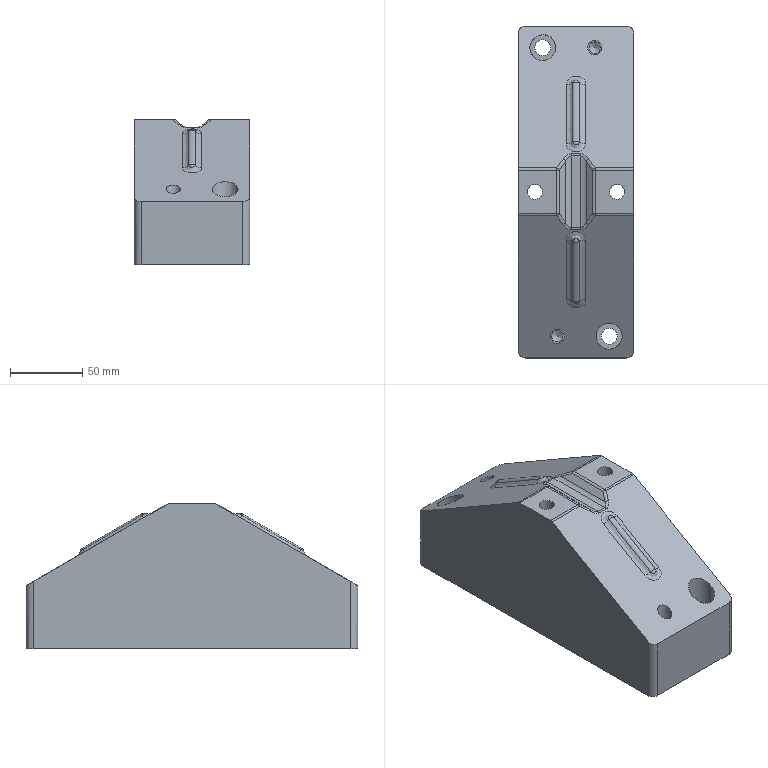Part | STEP file | 1_id82_x_t | 1 solid | 70 faces | box 80 x 230 x 101 mm | volume 1363447 mm3 | spline 24 | cylinder 22 | plane 14 | sphere 8 | cone 2 | commonest cylinder face diameters 10 x6 10.524 x4 6 x2 6.3 x2 7.938 x2 11 x2